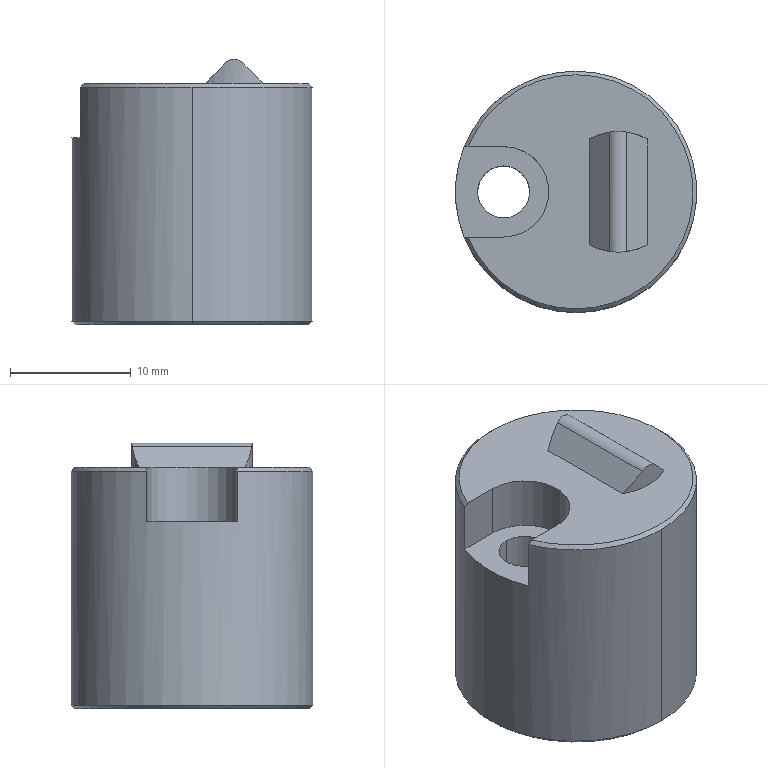Part | Creo | 1 solid | 18 faces | box 20 x 20 x 22 mm | volume 5882 mm3 | cylinder 8 | plane 7 | cone 3 | commonest cylinder face diameters 4.3 x2 10 x2 20 x2 2 x1 7.5 x1
STEP:
#1=CARTESIAN_POINT('',(181.054,116.245,-53.591));
#2=VERTEX_POINT('',#1);
#3=CARTESIAN_POINT('',(190.,129.695,-53.591));
#4=VERTEX_POINT('',#3);
#5=CARTESIAN_POINT('',(190.,119.995,-53.591));
#6=DIRECTION('',(0.,0.,1.));
#7=DIRECTION('',(-0.9222,-0.3866,0.));
#8=AXIS2_PLACEMENT_3D('',#5,#6,#7);
#9=CIRCLE('',#8,9.7);
#10=EDGE_CURVE('',#2,#4,#9,.T.);
#11=ORIENTED_EDGE('',*,*,#10,.F.);
#12=CARTESIAN_POINT('',(184.,116.245,-53.591));
#13=VERTEX_POINT('',#12);
#14=CARTESIAN_POINT('',(184.,116.245,-53.591));
#15=DIRECTION('',(-1.,0.,0.));
#16=VECTOR('',#15,2.946);
#17=LINE('',#14,#16);
#18=EDGE_CURVE('',#13,#2,#17,.T.);
#19=ORIENTED_EDGE('',*,*,#18,.F.);
#20=CARTESIAN_POINT('',(184.,123.745,-53.591));
#21=VERTEX_POINT('',#20);
#22=CARTESIAN_POINT('',(184.,119.995,-53.591));
#23=DIRECTION('',(0.,0.,-1.));
#24=DIRECTION('',(0.,1.,0.));
#25=AXIS2_PLACEMENT_3D('',#22,#23,#24);
#26=CIRCLE('',#25,3.75);
#27=EDGE_CURVE('',#21,#13,#26,.T.);
#28=ORIENTED_EDGE('',*,*,#27,.F.);
#29=CARTESIAN_POINT('',(181.054,123.745,-53.591));
#30=VERTEX_POINT('',#29);
#31=CARTESIAN_POINT('',(181.054,123.745,-53.591));
#32=DIRECTION('',(1.,0.,0.));
#33=VECTOR('',#32,2.946);
#34=LINE('',#31,#33);
#35=EDGE_CURVE('',#30,#21,#34,.T.);
#36=ORIENTED_EDGE('',*,*,#35,.F.);
#37=CARTESIAN_POINT('',(190.,119.995,-53.591));
#38=DIRECTION('',(0.,0.,1.));
#39=DIRECTION('',(0.,1.,0.));
#40=AXIS2_PLACEMENT_3D('',#37,#38,#39);
#41=CIRCLE('',#40,9.7);
#42=EDGE_CURVE('',#4,#30,#41,.T.);
#43=ORIENTED_EDGE('',*,*,#42,.F.);
#44=EDGE_LOOP('',(#11,#19,#28,#36,#43));
#45=FACE_OUTER_BOUND('',#44,.F.);
#46=CARTESIAN_POINT('',(195.914,115.617,-53.591));
#47=VERTEX_POINT('',#46);
#48=CARTESIAN_POINT('',(193.5,114.995,-53.591));
#49=VERTEX_POINT('',#48);
#50=CARTESIAN_POINT('',(193.5,119.995,-53.591));
#51=DIRECTION('',(0.,0.,-1.));
#52=DIRECTION('',(0.4828,-0.8757,0.));
#53=AXIS2_PLACEMENT_3D('',#50,#51,#52);
#54=CIRCLE('',#53,5.);
#55=EDGE_CURVE('',#47,#49,#54,.T.);
#56=ORIENTED_EDGE('',*,*,#55,.F.);
#57=CARTESIAN_POINT('',(195.914,124.374,-53.591));
#58=VERTEX_POINT('',#57);
#59=CARTESIAN_POINT('',(195.914,124.374,-53.591));
#60=DIRECTION('',(0.,-1.,0.));
#61=VECTOR('',#60,8.757);
#62=LINE('',#59,#61);
#63=EDGE_CURVE('',#58,#47,#62,.T.);
#64=ORIENTED_EDGE('',*,*,#63,.F.);
#65=CARTESIAN_POINT('',(193.5,124.995,-53.591));
#66=VERTEX_POINT('',#65);
#67=CARTESIAN_POINT('',(193.5,119.995,-53.591));
#68=DIRECTION('',(0.,0.,-1.));
#69=DIRECTION('',(0.,1.,0.));
#70=AXIS2_PLACEMENT_3D('',#67,#68,#69);
#71=CIRCLE('',#70,5.);
#72=EDGE_CURVE('',#66,#58,#71,.T.);
#73=ORIENTED_EDGE('',*,*,#72,.F.);
#74=CARTESIAN_POINT('',(191.086,124.374,-53.591));
#75=VERTEX_POINT('',#74);
#76=CARTESIAN_POINT('',(193.5,119.995,-53.591));
#77=DIRECTION('',(0.,0.,-1.));
#78=DIRECTION('',(-0.4828,0.8757,0.));
#79=AXIS2_PLACEMENT_3D('',#76,#77,#78);
#80=CIRCLE('',#79,5.);
#81=EDGE_CURVE('',#75,#66,#80,.T.);
#82=ORIENTED_EDGE('',*,*,#81,.F.);
#83=CARTESIAN_POINT('',(191.086,115.617,-53.591));
#84=VERTEX_POINT('',#83);
#85=CARTESIAN_POINT('',(191.086,124.374,-53.591));
#86=DIRECTION('',(0.,-1.,0.));
#87=VECTOR('',#86,8.757);
#88=LINE('',#85,#87);
#89=EDGE_CURVE('',#75,#84,#88,.T.);
#90=ORIENTED_EDGE('',*,*,#89,.T.);
#91=CARTESIAN_POINT('',(193.5,119.995,-53.591));
#92=DIRECTION('',(0.,0.,-1.));
#93=DIRECTION('',(0.,-1.,0.));
#94=AXIS2_PLACEMENT_3D('',#91,#92,#93);
#95=CIRCLE('',#94,5.);
#96=EDGE_CURVE('',#49,#84,#95,.T.);
#97=ORIENTED_EDGE('',*,*,#96,.F.);
#98=EDGE_LOOP('',(#56,#64,#73,#82,#90,#97));
#99=FACE_BOUND('',#98,.F.);
#100=CARTESIAN_POINT('',(190.,119.995,-53.591));
#101=DIRECTION('',(0.,0.,1.));
#102=DIRECTION('',(0.,-1.,0.));
#103=AXIS2_PLACEMENT_3D('',#100,#101,#102);
#104=PLANE('',#103);
#105=ADVANCED_FACE('',(#45,#99),#104,.T.);
#106=CARTESIAN_POINT('',(192.793,115.046,-51.884));
#107=VERTEX_POINT('',#106);
#108=CARTESIAN_POINT('',(192.206,115.129,-52.471));
#109=CARTESIAN_POINT('',(191.636,115.314,-53.041));
#110=CARTESIAN_POINT('',(191.086,115.617,-53.591));
#111=B_SPLINE_CURVE_WITH_KNOTS('',3,(#106,#108,#109,#110),.UNSPECIFIED.,.F.,.F.,(4,4),(0.,1.),.UNSPECIFIED.);
#112=EDGE_CURVE('',#107,#84,#111,.T.);
#113=ORIENTED_EDGE('',*,*,#112,.F.);
#114=CARTESIAN_POINT('',(194.207,115.046,-51.884));
#115=VERTEX_POINT('',#114);
#116=CARTESIAN_POINT('',(194.207,115.046,-51.884));
#117=CARTESIAN_POINT('',(194.153,115.038,-51.829));
#118=CARTESIAN_POINT('',(194.035,115.023,-51.736));
#119=CARTESIAN_POINT('',(193.831,115.005,-51.639));
#120=CARTESIAN_POINT('',(193.613,114.995,-51.589));
#121=CARTESIAN_POINT('',(193.389,114.995,-51.589));
#122=CARTESIAN_POINT('',(193.17,115.005,-51.638));
#123=CARTESIAN_POINT('',(192.966,115.023,-51.736));
#124=CARTESIAN_POINT('',(192.848,115.038,-51.829));
#125=CARTESIAN_POINT('',(192.793,115.046,-51.884));
#126=B_SPLINE_CURVE_WITH_KNOTS('',3,(#116,#117,#118,#119,#120,#121,#122,#123,#124,#125),.UNSPECIFIED.,.F.,.F.,(4,1,1,1,1,1,1,4),(0.,0.1429,0.2857,0.4286,0.5714,0.7143,0.8571,1.),.UNSPECIFIED.);
#127=EDGE_CURVE('',#115,#107,#126,.T.);
#128=ORIENTED_EDGE('',*,*,#127,.F.);
#129=CARTESIAN_POINT('',(195.914,115.617,-53.591));
#130=CARTESIAN_POINT('',(195.364,115.314,-53.041));
#131=CARTESIAN_POINT('',(194.794,115.129,-52.471));
#132=CARTESIAN_POINT('',(194.207,115.046,-51.884));
#133=B_SPLINE_CURVE_WITH_KNOTS('',3,(#129,#130,#131,#132),.UNSPECIFIED.,.F.,.F.,(4,4),(0.,1.),.UNSPECIFIED.);
#134=EDGE_CURVE('',#47,#115,#133,.T.);
#135=ORIENTED_EDGE('',*,*,#134,.F.);
#136=ORIENTED_EDGE('',*,*,#55,.T.);
#137=ORIENTED_EDGE('',*,*,#96,.T.);
#138=EDGE_LOOP('',(#113,#128,#135,#136,#137));
#139=FACE_OUTER_BOUND('',#138,.F.);
#140=CARTESIAN_POINT('',(193.5,119.995,-33.591));
#141=DIRECTION('',(0.,0.,-1.));
#142=DIRECTION('',(0.,1.,0.));
#143=AXIS2_PLACEMENT_3D('',#140,#141,#142);
#144=CYLINDRICAL_SURFACE('',#143,5.);
#145=ADVANCED_FACE('',(#139),#144,.T.);
#146=ORIENTED_EDGE('',*,*,#89,.F.);
#147=CARTESIAN_POINT('',(192.793,124.945,-51.884));
#148=VERTEX_POINT('',#147);
#149=CARTESIAN_POINT('',(191.086,124.374,-53.591));
#150=CARTESIAN_POINT('',(191.636,124.677,-53.041));
#151=CARTESIAN_POINT('',(192.206,124.861,-52.471));
#152=CARTESIAN_POINT('',(192.793,124.945,-51.884));
#153=B_SPLINE_CURVE_WITH_KNOTS('',3,(#149,#150,#151,#152),.UNSPECIFIED.,.F.,.F.,(4,4),(0.,1.),.UNSPECIFIED.);
#154=EDGE_CURVE('',#75,#148,#153,.T.);
#155=ORIENTED_EDGE('',*,*,#154,.T.);
#156=CARTESIAN_POINT('',(192.793,124.945,-51.884));
#157=DIRECTION('',(0.,-1.,0.));
#158=VECTOR('',#157,9.899);
#159=LINE('',#156,#158);
#160=EDGE_CURVE('',#148,#107,#159,.T.);
#161=ORIENTED_EDGE('',*,*,#160,.T.);
#162=ORIENTED_EDGE('',*,*,#112,.T.);
#163=EDGE_LOOP('',(#146,#155,#161,#162));
#164=FACE_OUTER_BOUND('',#163,.F.);
#165=CARTESIAN_POINT('',(192.793,114.995,-51.884));
#166=DIRECTION('',(0.7071,0.,-0.7071));
#167=DIRECTION('',(0.7071,0.,0.7071));
#168=AXIS2_PLACEMENT_3D('',#165,#166,#167);
#169=PLANE('',#168);
#170=ADVANCED_FACE('',(#164),#169,.F.);
#171=CARTESIAN_POINT('',(194.207,124.945,-51.884));
#172=VERTEX_POINT('',#171);
#173=CARTESIAN_POINT('',(194.794,124.861,-52.471));
#174=CARTESIAN_POINT('',(195.364,124.677,-53.041));
#175=CARTESIAN_POINT('',(195.914,124.374,-53.591));
#176=B_SPLINE_CURVE_WITH_KNOTS('',3,(#171,#173,#174,#175),.UNSPECIFIED.,.F.,.F.,(4,4),(0.,1.),.UNSPECIFIED.);
#177=EDGE_CURVE('',#172,#58,#176,.T.);
#178=ORIENTED_EDGE('',*,*,#177,.F.);
#179=CARTESIAN_POINT('',(193.5,124.995,-51.591));
#180=VERTEX_POINT('',#179);
#181=CARTESIAN_POINT('',(193.566,124.995,-51.591));
#182=CARTESIAN_POINT('',(193.695,124.993,-51.604));
#183=CARTESIAN_POINT('',(193.884,124.982,-51.66));
#184=CARTESIAN_POINT('',(194.059,124.965,-51.754));
#185=CARTESIAN_POINT('',(194.16,124.952,-51.837));
#186=CARTESIAN_POINT('',(194.207,124.945,-51.884));
#187=B_SPLINE_CURVE_WITH_KNOTS('',3,(#179,#181,#182,#183,#184,#185,#186),.UNSPECIFIED.,.F.,.F.,(4,1,1,1,4),(0.,0.25,0.5,0.75,1.),.UNSPECIFIED.);
#188=EDGE_CURVE('',#180,#172,#187,.T.);
#189=ORIENTED_EDGE('',*,*,#188,.F.);
#190=CARTESIAN_POINT('',(192.793,124.945,-51.884));
#191=CARTESIAN_POINT('',(192.84,124.952,-51.837));
#192=CARTESIAN_POINT('',(192.941,124.965,-51.754));
#193=CARTESIAN_POINT('',(193.116,124.982,-51.66));
#194=CARTESIAN_POINT('',(193.305,124.993,-51.604));
#195=CARTESIAN_POINT('',(193.434,124.995,-51.591));
#196=CARTESIAN_POINT('',(193.5,124.995,-51.591));
#197=B_SPLINE_CURVE_WITH_KNOTS('',3,(#190,#191,#192,#193,#194,#195,#196),.UNSPECIFIED.,.F.,.F.,(4,1,1,1,4),(0.,0.25,0.5,0.75,1.),.UNSPECIFIED.);
#198=EDGE_CURVE('',#148,#180,#197,.T.);
#199=ORIENTED_EDGE('',*,*,#198,.F.);
#200=ORIENTED_EDGE('',*,*,#154,.F.);
#201=ORIENTED_EDGE('',*,*,#81,.T.);
#202=ORIENTED_EDGE('',*,*,#72,.T.);
#203=EDGE_LOOP('',(#178,#189,#199,#200,#201,#202));
#204=FACE_OUTER_BOUND('',#203,.F.);
#205=CARTESIAN_POINT('',(193.5,119.995,-33.591));
#206=DIRECTION('',(0.,0.,-1.));
#207=DIRECTION('',(0.,1.,0.));
#208=AXIS2_PLACEMENT_3D('',#205,#206,#207);
#209=CYLINDRICAL_SURFACE('',#208,5.);
#210=ADVANCED_FACE('',(#204),#209,.T.);
#211=ORIENTED_EDGE('',*,*,#63,.T.);
#212=ORIENTED_EDGE('',*,*,#134,.T.);
#213=CARTESIAN_POINT('',(194.207,115.046,-51.884));
#214=DIRECTION('',(0.,1.,0.));
#215=VECTOR('',#214,9.899);
#216=LINE('',#213,#215);
#217=EDGE_CURVE('',#115,#172,#216,.T.);
#218=ORIENTED_EDGE('',*,*,#217,.T.);
#219=ORIENTED_EDGE('',*,*,#177,.T.);
#220=EDGE_LOOP('',(#211,#212,#218,#219));
#221=FACE_OUTER_BOUND('',#220,.F.);
#222=CARTESIAN_POINT('',(195.914,114.995,-53.591));
#223=DIRECTION('',(-0.7071,0.,-0.7071));
#224=DIRECTION('',(0.7071,0.,-0.7071));
#225=AXIS2_PLACEMENT_3D('',#222,#223,#224);
#226=PLANE('',#225);
#227=ADVANCED_FACE('',(#221),#226,.F.);
#228=ORIENTED_EDGE('',*,*,#217,.F.);
#229=ORIENTED_EDGE('',*,*,#127,.T.);
#230=ORIENTED_EDGE('',*,*,#160,.F.);
#231=ORIENTED_EDGE('',*,*,#198,.T.);
#232=ORIENTED_EDGE('',*,*,#188,.T.);
#233=EDGE_LOOP('',(#228,#229,#230,#231,#232));
#234=FACE_OUTER_BOUND('',#233,.F.);
#235=CARTESIAN_POINT('',(193.5,114.995,-52.591));
#236=DIRECTION('',(0.,1.,0.));
#237=DIRECTION('',(0.,0.,1.));
#238=AXIS2_PLACEMENT_3D('',#235,#236,#237);
#239=CYLINDRICAL_SURFACE('',#238,1.);
#240=ADVANCED_FACE('',(#234),#239,.T.);
#241=CARTESIAN_POINT('',(190.,109.995,-53.891));
#242=VERTEX_POINT('',#241);
#243=CARTESIAN_POINT('',(190.,129.995,-53.891));
#244=VERTEX_POINT('',#243);
#245=CARTESIAN_POINT('',(190.,119.995,-53.891));
#246=DIRECTION('',(0.,0.,1.));
#247=DIRECTION('',(0.,-1.,0.));
#248=AXIS2_PLACEMENT_3D('',#245,#246,#247);
#249=CIRCLE('',#248,10.);
#250=EDGE_CURVE('',#242,#244,#249,.T.);
#251=ORIENTED_EDGE('',*,*,#250,.F.);
#252=CARTESIAN_POINT('',(180.73,116.245,-53.891));
#253=VERTEX_POINT('',#252);
#254=CARTESIAN_POINT('',(190.,119.995,-53.891));
#255=DIRECTION('',(0.,0.,1.));
#256=DIRECTION('',(-0.927,-0.375,0.));
#257=AXIS2_PLACEMENT_3D('',#254,#255,#256);
#258=CIRCLE('',#257,10.);
#259=EDGE_CURVE('',#253,#242,#258,.T.);
#260=ORIENTED_EDGE('',*,*,#259,.F.);
#261=CARTESIAN_POINT('',(181.054,116.245,-53.591));
#262=CARTESIAN_POINT('',(181.018,116.245,-53.624));
#263=CARTESIAN_POINT('',(180.946,116.245,-53.691));
#264=CARTESIAN_POINT('',(180.838,116.245,-53.791));
#265=CARTESIAN_POINT('',(180.766,116.245,-53.858));
#266=B_SPLINE_CURVE_WITH_KNOTS('',3,(#261,#262,#263,#264,#265,#252),.UNSPECIFIED.,.F.,.F.,(4,1,1,4),(0.,0.3333,0.6667,1.),.UNSPECIFIED.);
#267=EDGE_CURVE('',#2,#253,#266,.T.);
#268=ORIENTED_EDGE('',*,*,#267,.F.);
#269=ORIENTED_EDGE('',*,*,#10,.T.);
#270=ORIENTED_EDGE('',*,*,#42,.T.);
#271=CARTESIAN_POINT('',(180.73,123.745,-53.891));
#272=VERTEX_POINT('',#271);
#273=CARTESIAN_POINT('',(180.766,123.745,-53.858));
#274=CARTESIAN_POINT('',(180.838,123.745,-53.791));
#275=CARTESIAN_POINT('',(180.946,123.745,-53.691));
#276=CARTESIAN_POINT('',(181.018,123.745,-53.624));
#277=CARTESIAN_POINT('',(181.054,123.745,-53.591));
#278=B_SPLINE_CURVE_WITH_KNOTS('',3,(#271,#273,#274,#275,#276,#277),.UNSPECIFIED.,.F.,.F.,(4,1,1,4),(0.,0.3333,0.6667,1.),.UNSPECIFIED.);
#279=EDGE_CURVE('',#272,#30,#278,.T.);
#280=ORIENTED_EDGE('',*,*,#279,.F.);
#281=CARTESIAN_POINT('',(190.,119.995,-53.891));
#282=DIRECTION('',(0.,0.,1.));
#283=DIRECTION('',(0.,1.,0.));
#284=AXIS2_PLACEMENT_3D('',#281,#282,#283);
#285=CIRCLE('',#284,10.);
#286=EDGE_CURVE('',#244,#272,#285,.T.);
#287=ORIENTED_EDGE('',*,*,#286,.F.);
#288=EDGE_LOOP('',(#251,#260,#268,#269,#270,#280,#287));
#289=FACE_OUTER_BOUND('',#288,.F.);
#290=CARTESIAN_POINT('',(190.,119.995,-53.741));
#291=DIRECTION('',(0.,0.,-1.));
#292=DIRECTION('',(0.,1.,0.));
#293=AXIS2_PLACEMENT_3D('',#290,#291,#292);
#294=CONICAL_SURFACE('',#293,9.85,45.);
#295=ADVANCED_FACE('',(#289),#294,.T.);
#296=ORIENTED_EDGE('',*,*,#250,.T.);
#297=CARTESIAN_POINT('',(190.,129.995,-73.291));
#298=VERTEX_POINT('',#297);
#299=CARTESIAN_POINT('',(190.,129.995,-73.291));
#300=DIRECTION('',(0.,0.,1.));
#301=VECTOR('',#300,19.4);
#302=LINE('',#299,#301);
#303=EDGE_CURVE('',#298,#244,#302,.T.);
#304=ORIENTED_EDGE('',*,*,#303,.F.);
#305=CARTESIAN_POINT('',(190.,109.995,-73.291));
#306=VERTEX_POINT('',#305);
#307=CARTESIAN_POINT('',(190.,119.995,-73.291));
#308=DIRECTION('',(0.,0.,-1.));
#309=DIRECTION('',(0.,1.,0.));
#310=AXIS2_PLACEMENT_3D('',#307,#308,#309);
#311=CIRCLE('',#310,10.);
#312=EDGE_CURVE('',#298,#306,#311,.T.);
#313=ORIENTED_EDGE('',*,*,#312,.T.);
#314=CARTESIAN_POINT('',(190.,109.995,-73.291));
#315=DIRECTION('',(0.,0.,1.));
#316=VECTOR('',#315,19.4);
#317=LINE('',#314,#316);
#318=EDGE_CURVE('',#306,#242,#317,.T.);
#319=ORIENTED_EDGE('',*,*,#318,.T.);
#320=EDGE_LOOP('',(#296,#304,#313,#319));
#321=FACE_OUTER_BOUND('',#320,.F.);
#322=CARTESIAN_POINT('',(190.,119.995,-73.591));
#323=DIRECTION('',(0.,0.,1.));
#324=DIRECTION('',(0.,-1.,0.));
#325=AXIS2_PLACEMENT_3D('',#322,#323,#324);
#326=CYLINDRICAL_SURFACE('',#325,10.);
#327=ADVANCED_FACE('',(#321),#326,.T.);
#328=CARTESIAN_POINT('',(180.73,123.745,-58.091));
#329=VERTEX_POINT('',#328);
#330=CARTESIAN_POINT('',(180.73,123.745,-58.091));
#331=DIRECTION('',(0.,0.,1.));
#332=VECTOR('',#331,4.2);
#333=LINE('',#330,#332);
#334=EDGE_CURVE('',#329,#272,#333,.T.);
#335=ORIENTED_EDGE('',*,*,#334,.F.);
#336=CARTESIAN_POINT('',(180.73,116.245,-58.091));
#337=VERTEX_POINT('',#336);
#338=CARTESIAN_POINT('',(190.,119.995,-58.091));
#339=DIRECTION('',(0.,0.,1.));
#340=DIRECTION('',(-0.927,0.375,0.));
#341=AXIS2_PLACEMENT_3D('',#338,#339,#340);
#342=CIRCLE('',#341,10.);
#343=EDGE_CURVE('',#329,#337,#342,.T.);
#344=ORIENTED_EDGE('',*,*,#343,.T.);
#345=CARTESIAN_POINT('',(180.73,116.245,-53.891));
#346=DIRECTION('',(0.,0.,-1.));
#347=VECTOR('',#346,4.2);
#348=LINE('',#345,#347);
#349=EDGE_CURVE('',#253,#337,#348,.T.);
#350=ORIENTED_EDGE('',*,*,#349,.F.);
#351=ORIENTED_EDGE('',*,*,#259,.T.);
#352=ORIENTED_EDGE('',*,*,#318,.F.);
#353=CARTESIAN_POINT('',(190.,119.995,-73.291));
#354=DIRECTION('',(0.,0.,-1.));
#355=DIRECTION('',(0.,-1.,0.));
#356=AXIS2_PLACEMENT_3D('',#353,#354,#355);
#357=CIRCLE('',#356,10.);
#358=EDGE_CURVE('',#306,#298,#357,.T.);
#359=ORIENTED_EDGE('',*,*,#358,.T.);
#360=ORIENTED_EDGE('',*,*,#303,.T.);
#361=ORIENTED_EDGE('',*,*,#286,.T.);
#362=EDGE_LOOP('',(#335,#344,#350,#351,#352,#359,#360,#361));
#363=FACE_OUTER_BOUND('',#362,.F.);
#364=CARTESIAN_POINT('',(190.,119.995,-73.591));
#365=DIRECTION('',(0.,0.,1.));
#366=DIRECTION('',(0.,-1.,0.));
#367=AXIS2_PLACEMENT_3D('',#364,#365,#366);
#368=CYLINDRICAL_SURFACE('',#367,10.);
#369=ADVANCED_FACE('',(#363),#368,.T.);
#370=ORIENTED_EDGE('',*,*,#334,.T.);
#371=ORIENTED_EDGE('',*,*,#279,.T.);
#372=ORIENTED_EDGE('',*,*,#35,.T.);
#373=CARTESIAN_POINT('',(184.,123.745,-58.091));
#374=VERTEX_POINT('',#373);
#375=CARTESIAN_POINT('',(184.,123.745,-53.591));
#376=DIRECTION('',(0.,0.,-1.));
#377=VECTOR('',#376,4.5);
#378=LINE('',#375,#377);
#379=EDGE_CURVE('',#21,#374,#378,.T.);
#380=ORIENTED_EDGE('',*,*,#379,.T.);
#381=CARTESIAN_POINT('',(184.,123.745,-58.091));
#382=DIRECTION('',(-1.,0.,0.));
#383=VECTOR('',#382,3.27);
#384=LINE('',#381,#383);
#385=EDGE_CURVE('',#374,#329,#384,.T.);
#386=ORIENTED_EDGE('',*,*,#385,.T.);
#387=EDGE_LOOP('',(#370,#371,#372,#380,#386));
#388=FACE_OUTER_BOUND('',#387,.F.);
#389=CARTESIAN_POINT('',(184.,123.745,-58.091));
#390=DIRECTION('',(0.,1.,0.));
#391=DIRECTION('',(-1.,0.,0.));
#392=AXIS2_PLACEMENT_3D('',#389,#390,#391);
#393=PLANE('',#392);
#394=ADVANCED_FACE('',(#388),#393,.F.);
#395=ORIENTED_EDGE('',*,*,#27,.T.);
#396=CARTESIAN_POINT('',(184.,116.245,-58.091));
#397=VERTEX_POINT('',#396);
#398=CARTESIAN_POINT('',(184.,116.245,-58.091));
#399=DIRECTION('',(0.,0.,1.));
#400=VECTOR('',#399,4.5);
#401=LINE('',#398,#400);
#402=EDGE_CURVE('',#397,#13,#401,.T.);
#403=ORIENTED_EDGE('',*,*,#402,.F.);
#404=CARTESIAN_POINT('',(184.,119.995,-58.091));
#405=DIRECTION('',(0.,0.,1.));
#406=DIRECTION('',(0.,-1.,0.));
#407=AXIS2_PLACEMENT_3D('',#404,#405,#406);
#408=CIRCLE('',#407,3.75);
#409=EDGE_CURVE('',#397,#374,#408,.T.);
#410=ORIENTED_EDGE('',*,*,#409,.T.);
#411=ORIENTED_EDGE('',*,*,#379,.F.);
#412=EDGE_LOOP('',(#395,#403,#410,#411));
#413=FACE_OUTER_BOUND('',#412,.F.);
#414=CARTESIAN_POINT('',(184.,119.995,-53.591));
#415=DIRECTION('',(0.,0.,-1.));
#416=DIRECTION('',(0.,1.,0.));
#417=AXIS2_PLACEMENT_3D('',#414,#415,#416);
#418=CYLINDRICAL_SURFACE('',#417,3.75);
#419=ADVANCED_FACE('',(#413),#418,.F.);
#420=ORIENTED_EDGE('',*,*,#349,.T.);
#421=CARTESIAN_POINT('',(180.73,116.245,-58.091));
#422=DIRECTION('',(1.,0.,0.));
#423=VECTOR('',#422,3.27);
#424=LINE('',#421,#423);
#425=EDGE_CURVE('',#337,#397,#424,.T.);
#426=ORIENTED_EDGE('',*,*,#425,.T.);
#427=ORIENTED_EDGE('',*,*,#402,.T.);
#428=ORIENTED_EDGE('',*,*,#18,.T.);
#429=ORIENTED_EDGE('',*,*,#267,.T.);
#430=EDGE_LOOP('',(#420,#426,#427,#428,#429));
#431=FACE_OUTER_BOUND('',#430,.F.);
#432=CARTESIAN_POINT('',(176.5,116.245,-58.091));
#433=DIRECTION('',(0.,-1.,0.));
#434=DIRECTION('',(1.,0.,0.));
#435=AXIS2_PLACEMENT_3D('',#432,#433,#434);
#436=PLANE('',#435);
#437=ADVANCED_FACE('',(#431),#436,.F.);
#438=ORIENTED_EDGE('',*,*,#409,.F.);
#439=ORIENTED_EDGE('',*,*,#425,.F.);
#440=ORIENTED_EDGE('',*,*,#343,.F.);
#441=ORIENTED_EDGE('',*,*,#385,.F.);
#442=EDGE_LOOP('',(#438,#439,#440,#441));
#443=FACE_OUTER_BOUND('',#442,.F.);
#444=CARTESIAN_POINT('',(184.,122.145,-58.091));
#445=VERTEX_POINT('',#444);
#446=CARTESIAN_POINT('',(184.,117.845,-58.091));
#447=VERTEX_POINT('',#446);
#448=CARTESIAN_POINT('',(184.,119.995,-58.091));
#449=DIRECTION('',(0.,0.,-1.));
#450=DIRECTION('',(0.,1.,0.));
#451=AXIS2_PLACEMENT_3D('',#448,#449,#450);
#452=CIRCLE('',#451,2.15);
#453=EDGE_CURVE('',#445,#447,#452,.T.);
#454=ORIENTED_EDGE('',*,*,#453,.F.);
#455=CARTESIAN_POINT('',(184.,119.995,-58.091));
#456=DIRECTION('',(0.,0.,-1.));
#457=DIRECTION('',(0.,-1.,0.));
#458=AXIS2_PLACEMENT_3D('',#455,#456,#457);
#459=CIRCLE('',#458,2.15);
#460=EDGE_CURVE('',#447,#445,#459,.T.);
#461=ORIENTED_EDGE('',*,*,#460,.F.);
#462=EDGE_LOOP('',(#454,#461));
#463=FACE_BOUND('',#462,.F.);
#464=CARTESIAN_POINT('',(190.,119.995,-58.091));
#465=DIRECTION('',(0.,0.,1.));
#466=DIRECTION('',(0.,-1.,0.));
#467=AXIS2_PLACEMENT_3D('',#464,#465,#466);
#468=PLANE('',#467);
#469=ADVANCED_FACE('',(#443,#463),#468,.T.);
#470=ORIENTED_EDGE('',*,*,#453,.T.);
#471=CARTESIAN_POINT('',(184.,117.845,-73.591));
#472=VERTEX_POINT('',#471);
#473=CARTESIAN_POINT('',(184.,117.845,-58.091));
#474=DIRECTION('',(0.,0.,-1.));
#475=VECTOR('',#474,15.5);
#476=LINE('',#473,#475);
#477=EDGE_CURVE('',#447,#472,#476,.T.);
#478=ORIENTED_EDGE('',*,*,#477,.T.);
#479=CARTESIAN_POINT('',(184.,122.145,-73.591));
#480=VERTEX_POINT('',#479);
#481=CARTESIAN_POINT('',(184.,119.995,-73.591));
#482=DIRECTION('',(0.,0.,1.));
#483=DIRECTION('',(0.,-1.,0.));
#484=AXIS2_PLACEMENT_3D('',#481,#482,#483);
#485=CIRCLE('',#484,2.15);
#486=EDGE_CURVE('',#472,#480,#485,.T.);
#487=ORIENTED_EDGE('',*,*,#486,.T.);
#488=CARTESIAN_POINT('',(184.,122.145,-58.091));
#489=DIRECTION('',(0.,0.,-1.));
#490=VECTOR('',#489,15.5);
#491=LINE('',#488,#490);
#492=EDGE_CURVE('',#445,#480,#491,.T.);
#493=ORIENTED_EDGE('',*,*,#492,.F.);
#494=EDGE_LOOP('',(#470,#478,#487,#493));
#495=FACE_OUTER_BOUND('',#494,.F.);
#496=CARTESIAN_POINT('',(184.,119.995,-53.591));
#497=DIRECTION('',(0.,0.,-1.));
#498=DIRECTION('',(0.,1.,0.));
#499=AXIS2_PLACEMENT_3D('',#496,#497,#498);
#500=CYLINDRICAL_SURFACE('',#499,2.15);
#501=ADVANCED_FACE('',(#495),#500,.F.);
#502=ORIENTED_EDGE('',*,*,#460,.T.);
#503=ORIENTED_EDGE('',*,*,#492,.T.);
#504=CARTESIAN_POINT('',(184.,119.995,-73.591));
#505=DIRECTION('',(0.,0.,1.));
#506=DIRECTION('',(0.,1.,0.));
#507=AXIS2_PLACEMENT_3D('',#504,#505,#506);
#508=CIRCLE('',#507,2.15);
#509=EDGE_CURVE('',#480,#472,#508,.T.);
#510=ORIENTED_EDGE('',*,*,#509,.T.);
#511=ORIENTED_EDGE('',*,*,#477,.F.);
#512=EDGE_LOOP('',(#502,#503,#510,#511));
#513=FACE_OUTER_BOUND('',#512,.F.);
#514=CARTESIAN_POINT('',(184.,119.995,-53.591));
#515=DIRECTION('',(0.,0.,-1.));
#516=DIRECTION('',(0.,1.,0.));
#517=AXIS2_PLACEMENT_3D('',#514,#515,#516);
#518=CYLINDRICAL_SURFACE('',#517,2.15);
#519=ADVANCED_FACE('',(#513),#518,.F.);
#520=CARTESIAN_POINT('',(190.,110.295,-73.591));
#521=VERTEX_POINT('',#520);
#522=CARTESIAN_POINT('',(190.,129.695,-73.591));
#523=VERTEX_POINT('',#522);
#524=CARTESIAN_POINT('',(190.,119.995,-73.591));
#525=DIRECTION('',(0.,0.,-1.));
#526=DIRECTION('',(0.,-1.,0.));
#527=AXIS2_PLACEMENT_3D('',#524,#525,#526);
#528=CIRCLE('',#527,9.7);
#529=EDGE_CURVE('',#521,#523,#528,.T.);
#530=ORIENTED_EDGE('',*,*,#529,.F.);
#531=CARTESIAN_POINT('',(190.,119.995,-73.591));
#532=DIRECTION('',(0.,0.,-1.));
#533=DIRECTION('',(0.,1.,0.));
#534=AXIS2_PLACEMENT_3D('',#531,#532,#533);
#535=CIRCLE('',#534,9.7);
#536=EDGE_CURVE('',#523,#521,#535,.T.);
#537=ORIENTED_EDGE('',*,*,#536,.F.);
#538=EDGE_LOOP('',(#530,#537));
#539=FACE_OUTER_BOUND('',#538,.F.);
#540=ORIENTED_EDGE('',*,*,#509,.F.);
#541=ORIENTED_EDGE('',*,*,#486,.F.);
#542=EDGE_LOOP('',(#540,#541));
#543=FACE_BOUND('',#542,.F.);
#544=CARTESIAN_POINT('',(190.,119.995,-73.591));
#545=DIRECTION('',(0.,0.,1.));
#546=DIRECTION('',(0.,-1.,0.));
#547=AXIS2_PLACEMENT_3D('',#544,#545,#546);
#548=PLANE('',#547);
#549=ADVANCED_FACE('',(#539,#543),#548,.F.);
#550=ORIENTED_EDGE('',*,*,#529,.T.);
#551=CARTESIAN_POINT('',(190.,129.695,-73.591));
#552=DIRECTION('',(0.,0.7071,0.7071));
#553=VECTOR('',#552,0.4243);
#554=LINE('',#551,#553);
#555=EDGE_CURVE('',#523,#298,#554,.T.);
#556=ORIENTED_EDGE('',*,*,#555,.T.);
#557=ORIENTED_EDGE('',*,*,#358,.F.);
#558=CARTESIAN_POINT('',(190.,110.295,-73.591));
#559=DIRECTION('',(0.,-0.7071,0.7071));
#560=VECTOR('',#559,0.4243);
#561=LINE('',#558,#560);
#562=EDGE_CURVE('',#521,#306,#561,.T.);
#563=ORIENTED_EDGE('',*,*,#562,.F.);
#564=EDGE_LOOP('',(#550,#556,#557,#563));
#565=FACE_OUTER_BOUND('',#564,.F.);
#566=CARTESIAN_POINT('',(190.,119.995,-73.441));
#567=DIRECTION('',(0.,0.,1.));
#568=DIRECTION('',(0.,-1.,0.));
#569=AXIS2_PLACEMENT_3D('',#566,#567,#568);
#570=CONICAL_SURFACE('',#569,9.85,45.);
#571=ADVANCED_FACE('',(#565),#570,.T.);
#572=ORIENTED_EDGE('',*,*,#536,.T.);
#573=ORIENTED_EDGE('',*,*,#562,.T.);
#574=ORIENTED_EDGE('',*,*,#312,.F.);
#575=ORIENTED_EDGE('',*,*,#555,.F.);
#576=EDGE_LOOP('',(#572,#573,#574,#575));
#577=FACE_OUTER_BOUND('',#576,.F.);
#578=CARTESIAN_POINT('',(190.,119.995,-73.441));
#579=DIRECTION('',(0.,0.,1.));
#580=DIRECTION('',(0.,-1.,0.));
#581=AXIS2_PLACEMENT_3D('',#578,#579,#580);
#582=CONICAL_SURFACE('',#581,9.85,45.);
#583=ADVANCED_FACE('',(#577),#582,.T.);
#584=CLOSED_SHELL('',(#105,#145,#170,#210,#227,#240,#295,#327,#369,#394,#419,#437,#469,#501,#519,#549,#571,#583));
#585=MANIFOLD_SOLID_BREP('',#584);
#586=(LENGTH_UNIT()NAMED_UNIT(*)SI_UNIT(.MILLI.,.METRE.));
#587=UNCERTAINTY_MEASURE_WITH_UNIT(LENGTH_MEASURE(0.003583),#586,'','');
#588=(NAMED_UNIT(*)PLANE_ANGLE_UNIT()SI_UNIT($,.RADIAN.));
#589=PLANE_ANGLE_MEASURE_WITH_UNIT(PLANE_ANGLE_MEASURE(0.01745),#588);
#590=(CONVERSION_BASED_UNIT('DEGREE',#589)NAMED_UNIT(*)PLANE_ANGLE_UNIT());
#591=(NAMED_UNIT(*)SI_UNIT($,.STERADIAN.)SOLID_ANGLE_UNIT());
#592=(GEOMETRIC_REPRESENTATION_CONTEXT(3)GLOBAL_UNCERTAINTY_ASSIGNED_CONTEXT((#587))GLOBAL_UNIT_ASSIGNED_CONTEXT((#586,#590,#591))REPRESENTATION_CONTEXT('',''));
#593=ADVANCED_BREP_SHAPE_REPRESENTATION('',(#585),#592);